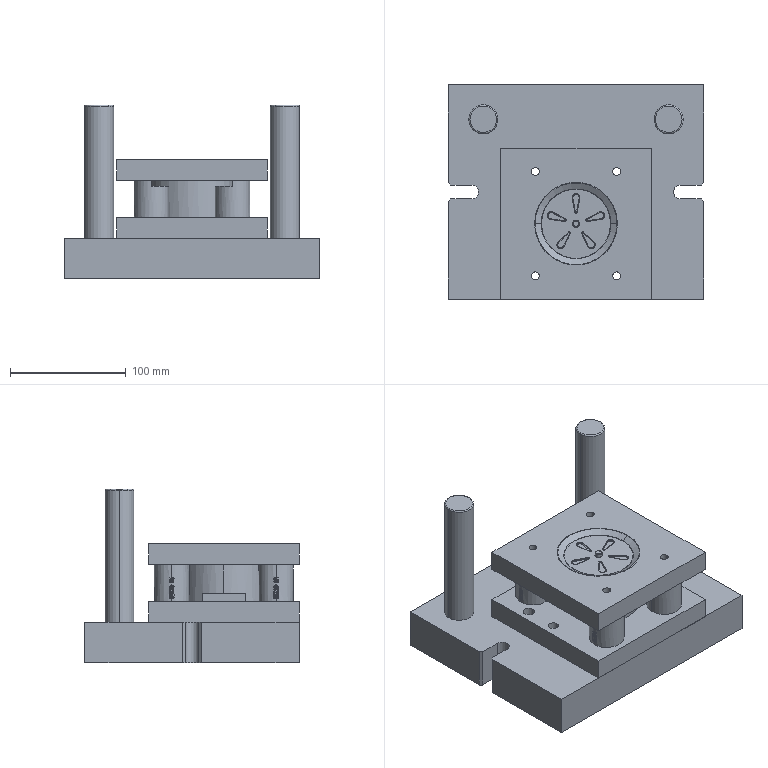Part | SolidWorks | 13 solids | 388 faces | box 220 x 185 x 150 mm | volume 2240435 mm3 | cylinder 233 | plane 91 | spline 30 | cone 26 | torus 8 | commonest cylinder face diameters 30 x136 6.806 x12 14.5 x12 10 x10 9 x8 15.003 x8